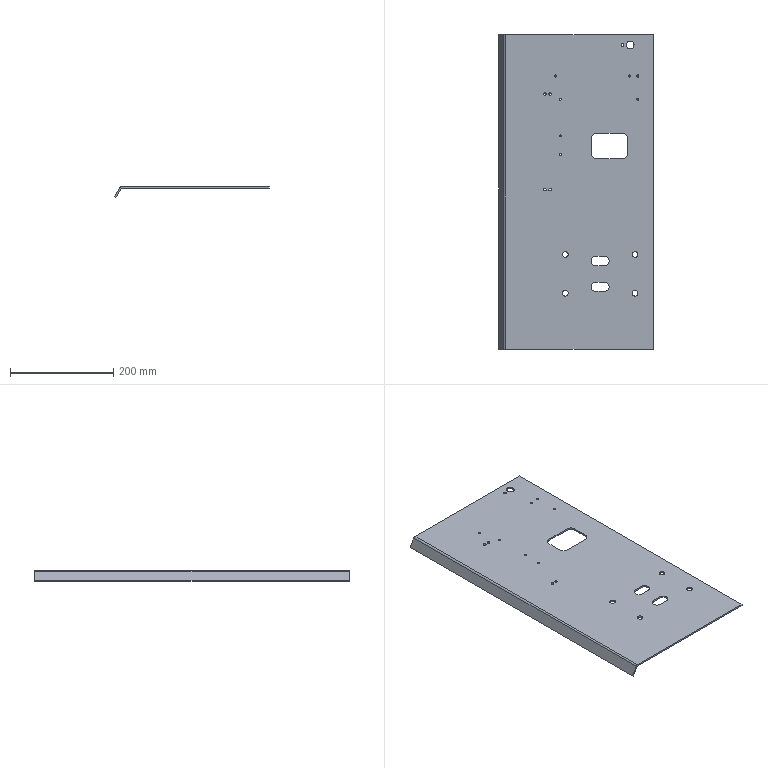Part | STEP file | PN_0024_default | 1 solid | 47 faces | box 299.634 x 609 x 21.187 mm | volume 548707 mm3 | cylinder 27 | plane 20 | commonest cylinder face diameters 4 x7 5 x5 11 x4 18 x4 20 x4 2 x1